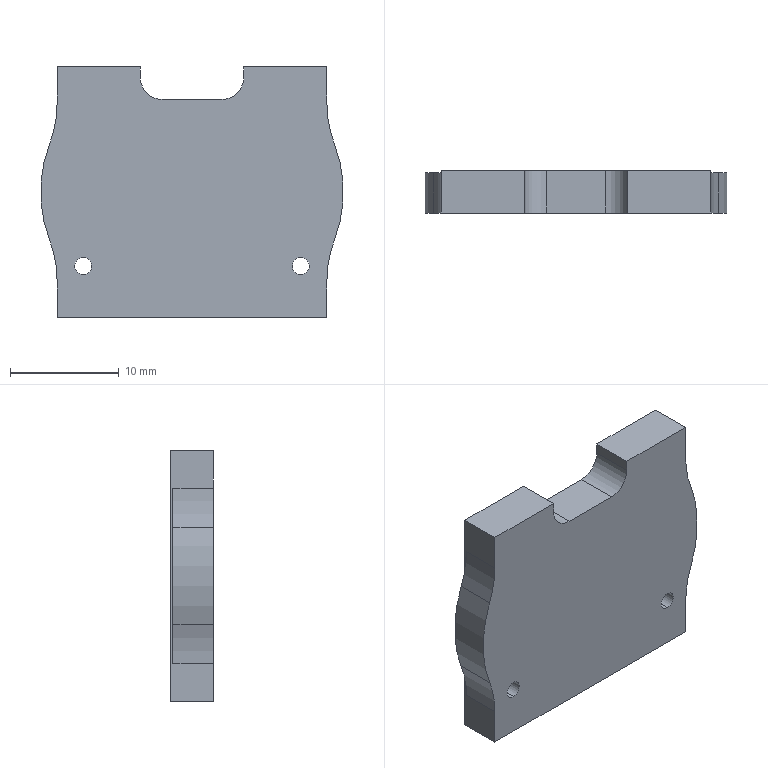Part | SolidWorks | features BaseBody 1 | 1 solid | 121 faces | box 27.8 x 3.9 x 23 mm | volume 2196 mm3 | plane 109 | cylinder 12 | commonest cylinder face diameters 1.567 x4 20 x4 4 x2 25 x2